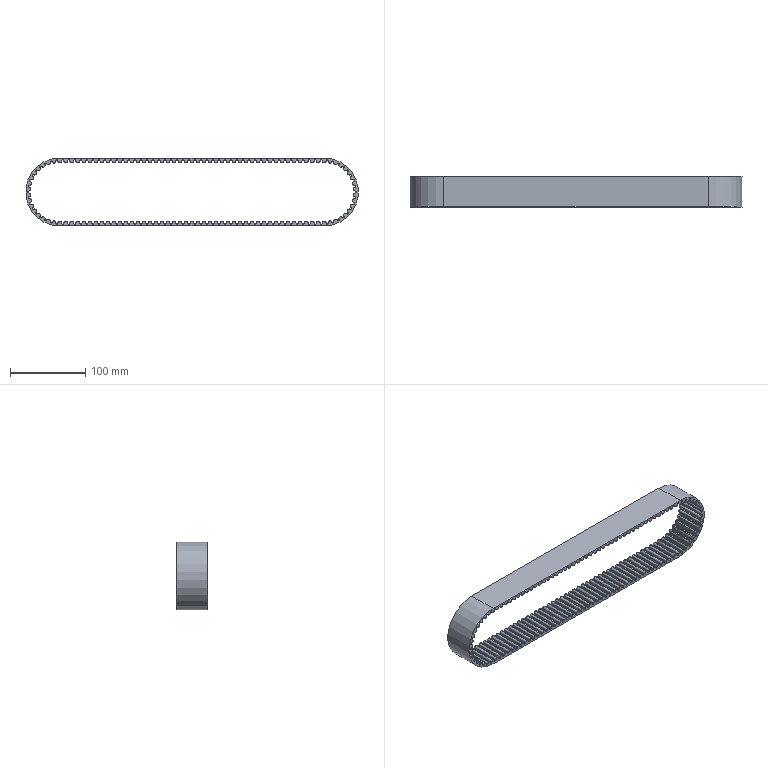Part | SolidWorks | features BaseBody 1 | 1 solid | 1044 faces | box 442.448 x 40 x 90.448 mm | volume 174219 mm3 | plane 526 | cylinder 518 | commonest cylinder face diameters 1.5 x258 4.92 x258 90.448 x2